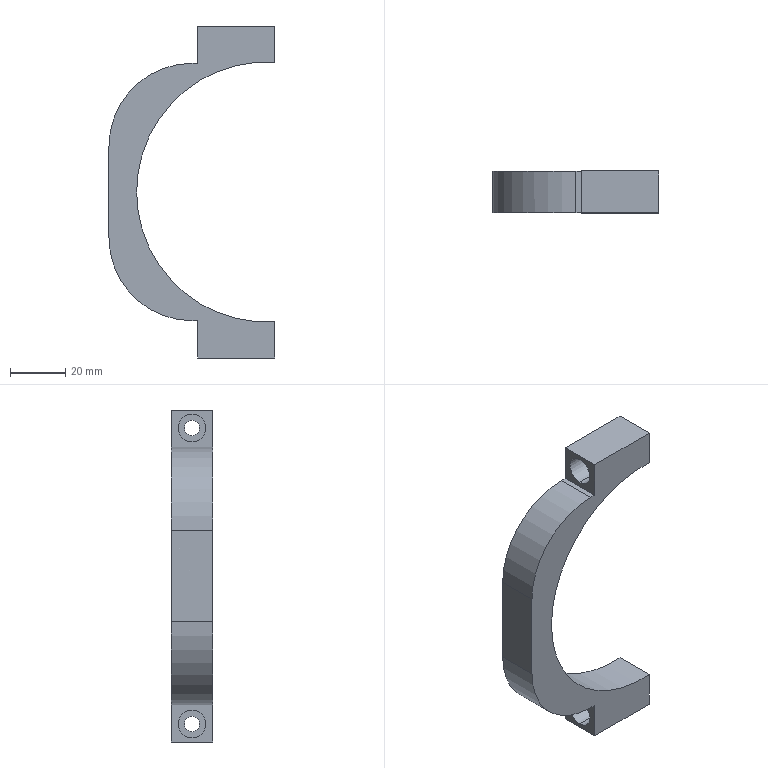Part | STEP file | 11-FG-S01311 | 1 solid | 25 faces | box 60 x 15 x 120 mm | volume 30172 mm3 | plane 13 | cylinder 12 | commonest cylinder face diameters 5.5 x4 10 x4 60 x2 94 x2
STEP:
#1=CARTESIAN_POINT('',(-14.6,7.5,1.5));
#2=VERTEX_POINT('',#1);
#3=CARTESIAN_POINT('',(-14.6,7.5,11.5));
#4=VERTEX_POINT('',#3);
#5=CARTESIAN_POINT('',(-14.6,7.5,6.5));
#6=DIRECTION('',(-1.,0.,0.));
#7=DIRECTION('',(0.,0.,1.));
#8=AXIS2_PLACEMENT_3D('',#5,#6,#7);
#9=CIRCLE('',#8,5.);
#10=EDGE_CURVE('',#2,#4,#9,.T.);
#11=ORIENTED_EDGE('',*,*,#10,.F.);
#12=CARTESIAN_POINT('',(-28.,7.5,1.5));
#13=VERTEX_POINT('',#12);
#14=CARTESIAN_POINT('',(-60.,7.5,1.5));
#15=DIRECTION('',(-1.,0.,0.));
#16=VECTOR('',#15,1000.);
#17=LINE('',#14,#16);
#18=EDGE_CURVE('',#2,#13,#17,.T.);
#19=ORIENTED_EDGE('',*,*,#18,.T.);
#20=CARTESIAN_POINT('',(-28.,7.5,11.5));
#21=VERTEX_POINT('',#20);
#22=CARTESIAN_POINT('',(-28.,7.5,6.5));
#23=DIRECTION('',(-1.,0.,0.));
#24=DIRECTION('',(0.,1.,0.));
#25=AXIS2_PLACEMENT_3D('',#22,#23,#24);
#26=CIRCLE('',#25,5.);
#27=EDGE_CURVE('',#13,#21,#26,.T.);
#28=ORIENTED_EDGE('',*,*,#27,.T.);
#29=CARTESIAN_POINT('',(-60.,7.5,11.5));
#30=DIRECTION('',(-1.,0.,0.));
#31=VECTOR('',#30,1000.);
#32=LINE('',#29,#31);
#33=EDGE_CURVE('',#4,#21,#32,.T.);
#34=ORIENTED_EDGE('',*,*,#33,.F.);
#35=EDGE_LOOP('',(#11,#19,#28,#34));
#36=FACE_OUTER_BOUND('',#35,.T.);
#37=CARTESIAN_POINT('',(-60.,7.5,6.5));
#38=DIRECTION('',(-1.,0.,0.));
#39=DIRECTION('',(0.,0.,1.));
#40=AXIS2_PLACEMENT_3D('',#37,#38,#39);
#41=CYLINDRICAL_SURFACE('',#40,5.);
#42=ADVANCED_FACE('',(#36),#41,.F.);
#43=CARTESIAN_POINT('',(0.,7.5,3.75));
#44=VERTEX_POINT('',#43);
#45=CARTESIAN_POINT('',(0.,7.5,9.25));
#46=VERTEX_POINT('',#45);
#47=CARTESIAN_POINT('',(0.,7.5,6.5));
#48=DIRECTION('',(-1.,0.,0.));
#49=DIRECTION('',(0.,0.,1.));
#50=AXIS2_PLACEMENT_3D('',#47,#48,#49);
#51=CIRCLE('',#50,2.75);
#52=EDGE_CURVE('',#44,#46,#51,.T.);
#53=ORIENTED_EDGE('',*,*,#52,.F.);
#54=CARTESIAN_POINT('',(-14.6,7.5,3.75));
#55=VERTEX_POINT('',#54);
#56=CARTESIAN_POINT('',(-60.,7.5,3.75));
#57=DIRECTION('',(-1.,0.,0.));
#58=VECTOR('',#57,1000.);
#59=LINE('',#56,#58);
#60=EDGE_CURVE('',#44,#55,#59,.T.);
#61=ORIENTED_EDGE('',*,*,#60,.T.);
#62=CARTESIAN_POINT('',(-14.6,7.5,9.25));
#63=VERTEX_POINT('',#62);
#64=CARTESIAN_POINT('',(-14.6,7.5,6.5));
#65=DIRECTION('',(-1.,0.,0.));
#66=DIRECTION('',(0.,0.,1.));
#67=AXIS2_PLACEMENT_3D('',#64,#65,#66);
#68=CIRCLE('',#67,2.75);
#69=EDGE_CURVE('',#55,#63,#68,.T.);
#70=ORIENTED_EDGE('',*,*,#69,.T.);
#71=CARTESIAN_POINT('',(-60.,7.5,9.25));
#72=DIRECTION('',(-1.,0.,0.));
#73=VECTOR('',#72,1000.);
#74=LINE('',#71,#73);
#75=EDGE_CURVE('',#46,#63,#74,.T.);
#76=ORIENTED_EDGE('',*,*,#75,.F.);
#77=EDGE_LOOP('',(#53,#61,#70,#76));
#78=FACE_OUTER_BOUND('',#77,.T.);
#79=CARTESIAN_POINT('',(-60.,7.5,6.5));
#80=DIRECTION('',(-1.,0.,0.));
#81=DIRECTION('',(0.,0.,1.));
#82=AXIS2_PLACEMENT_3D('',#79,#80,#81);
#83=CYLINDRICAL_SURFACE('',#82,2.75);
#84=ADVANCED_FACE('',(#78),#83,.F.);
#85=CARTESIAN_POINT('',(-14.6,7.5,108.5));
#86=VERTEX_POINT('',#85);
#87=CARTESIAN_POINT('',(-14.6,7.5,118.5));
#88=VERTEX_POINT('',#87);
#89=CARTESIAN_POINT('',(-14.6,7.5,113.5));
#90=DIRECTION('',(-1.,0.,0.));
#91=DIRECTION('',(0.,0.,1.));
#92=AXIS2_PLACEMENT_3D('',#89,#90,#91);
#93=CIRCLE('',#92,5.);
#94=EDGE_CURVE('',#86,#88,#93,.T.);
#95=ORIENTED_EDGE('',*,*,#94,.F.);
#96=CARTESIAN_POINT('',(-28.,7.5,108.5));
#97=VERTEX_POINT('',#96);
#98=CARTESIAN_POINT('',(-60.,7.5,108.5));
#99=DIRECTION('',(-1.,0.,0.));
#100=VECTOR('',#99,1000.);
#101=LINE('',#98,#100);
#102=EDGE_CURVE('',#86,#97,#101,.T.);
#103=ORIENTED_EDGE('',*,*,#102,.T.);
#104=CARTESIAN_POINT('',(-28.,7.5,118.5));
#105=VERTEX_POINT('',#104);
#106=CARTESIAN_POINT('',(-28.,7.5,113.5));
#107=DIRECTION('',(-1.,0.,0.));
#108=DIRECTION('',(0.,1.,0.));
#109=AXIS2_PLACEMENT_3D('',#106,#107,#108);
#110=CIRCLE('',#109,5.);
#111=EDGE_CURVE('',#97,#105,#110,.T.);
#112=ORIENTED_EDGE('',*,*,#111,.T.);
#113=CARTESIAN_POINT('',(-60.,7.5,118.5));
#114=DIRECTION('',(-1.,0.,0.));
#115=VECTOR('',#114,1000.);
#116=LINE('',#113,#115);
#117=EDGE_CURVE('',#88,#105,#116,.T.);
#118=ORIENTED_EDGE('',*,*,#117,.F.);
#119=EDGE_LOOP('',(#95,#103,#112,#118));
#120=FACE_OUTER_BOUND('',#119,.T.);
#121=CARTESIAN_POINT('',(-60.,7.5,113.5));
#122=DIRECTION('',(-1.,0.,0.));
#123=DIRECTION('',(0.,0.,1.));
#124=AXIS2_PLACEMENT_3D('',#121,#122,#123);
#125=CYLINDRICAL_SURFACE('',#124,5.);
#126=ADVANCED_FACE('',(#120),#125,.F.);
#127=CARTESIAN_POINT('',(0.,7.5,110.75));
#128=VERTEX_POINT('',#127);
#129=CARTESIAN_POINT('',(0.,7.5,116.25));
#130=VERTEX_POINT('',#129);
#131=CARTESIAN_POINT('',(0.,7.5,113.5));
#132=DIRECTION('',(-1.,0.,0.));
#133=DIRECTION('',(0.,0.,1.));
#134=AXIS2_PLACEMENT_3D('',#131,#132,#133);
#135=CIRCLE('',#134,2.75);
#136=EDGE_CURVE('',#128,#130,#135,.T.);
#137=ORIENTED_EDGE('',*,*,#136,.F.);
#138=CARTESIAN_POINT('',(-14.6,7.5,110.75));
#139=VERTEX_POINT('',#138);
#140=CARTESIAN_POINT('',(-60.,7.5,110.75));
#141=DIRECTION('',(-1.,0.,0.));
#142=VECTOR('',#141,1000.);
#143=LINE('',#140,#142);
#144=EDGE_CURVE('',#128,#139,#143,.T.);
#145=ORIENTED_EDGE('',*,*,#144,.T.);
#146=CARTESIAN_POINT('',(-14.6,7.5,116.25));
#147=VERTEX_POINT('',#146);
#148=CARTESIAN_POINT('',(-14.6,7.5,113.5));
#149=DIRECTION('',(-1.,0.,0.));
#150=DIRECTION('',(0.,0.,1.));
#151=AXIS2_PLACEMENT_3D('',#148,#149,#150);
#152=CIRCLE('',#151,2.75);
#153=EDGE_CURVE('',#139,#147,#152,.T.);
#154=ORIENTED_EDGE('',*,*,#153,.T.);
#155=CARTESIAN_POINT('',(-60.,7.5,116.25));
#156=DIRECTION('',(-1.,0.,0.));
#157=VECTOR('',#156,1000.);
#158=LINE('',#155,#157);
#159=EDGE_CURVE('',#130,#147,#158,.T.);
#160=ORIENTED_EDGE('',*,*,#159,.F.);
#161=EDGE_LOOP('',(#137,#145,#154,#160));
#162=FACE_OUTER_BOUND('',#161,.T.);
#163=CARTESIAN_POINT('',(-60.,7.5,113.5));
#164=DIRECTION('',(-1.,0.,0.));
#165=DIRECTION('',(0.,0.,1.));
#166=AXIS2_PLACEMENT_3D('',#163,#164,#165);
#167=CYLINDRICAL_SURFACE('',#166,2.75);
#168=ADVANCED_FACE('',(#162),#167,.F.);
#169=CARTESIAN_POINT('',(-50.,0.,60.));
#170=VERTEX_POINT('',#169);
#171=CARTESIAN_POINT('',(0.,0.,106.904));
#172=VERTEX_POINT('',#171);
#173=CARTESIAN_POINT('',(-3.,0.,60.));
#174=DIRECTION('',(0.,1.,0.));
#175=DIRECTION('',(-1.,0.,0.));
#176=AXIS2_PLACEMENT_3D('',#173,#174,#175);
#177=CIRCLE('',#176,47.);
#178=EDGE_CURVE('',#170,#172,#177,.T.);
#179=ORIENTED_EDGE('',*,*,#178,.F.);
#180=CARTESIAN_POINT('',(-50.,15.,60.));
#181=VERTEX_POINT('',#180);
#182=CARTESIAN_POINT('',(-50.,-65.,60.));
#183=DIRECTION('',(0.,1.,0.));
#184=VECTOR('',#183,1000.);
#185=LINE('',#182,#184);
#186=EDGE_CURVE('',#170,#181,#185,.T.);
#187=ORIENTED_EDGE('',*,*,#186,.T.);
#188=CARTESIAN_POINT('',(0.,15.,106.904));
#189=VERTEX_POINT('',#188);
#190=CARTESIAN_POINT('',(-3.,15.,60.));
#191=DIRECTION('',(0.,1.,0.));
#192=DIRECTION('',(-1.,0.,0.));
#193=AXIS2_PLACEMENT_3D('',#190,#191,#192);
#194=CIRCLE('',#193,47.);
#195=EDGE_CURVE('',#181,#189,#194,.T.);
#196=ORIENTED_EDGE('',*,*,#195,.T.);
#197=CARTESIAN_POINT('',(0.,-65.,106.904));
#198=DIRECTION('',(0.,1.,0.));
#199=VECTOR('',#198,1000.);
#200=LINE('',#197,#199);
#201=EDGE_CURVE('',#172,#189,#200,.T.);
#202=ORIENTED_EDGE('',*,*,#201,.F.);
#203=EDGE_LOOP('',(#179,#187,#196,#202));
#204=FACE_OUTER_BOUND('',#203,.T.);
#205=CARTESIAN_POINT('',(-3.,-65.,60.));
#206=DIRECTION('',(0.,1.,0.));
#207=DIRECTION('',(-1.,0.,0.));
#208=AXIS2_PLACEMENT_3D('',#205,#206,#207);
#209=CYLINDRICAL_SURFACE('',#208,47.);
#210=ADVANCED_FACE('',(#204),#209,.F.);
#211=CARTESIAN_POINT('',(0.,7.5,113.5));
#212=DIRECTION('',(-1.,0.,0.));
#213=DIRECTION('',(0.,0.,1.));
#214=AXIS2_PLACEMENT_3D('',#211,#212,#213);
#215=CIRCLE('',#214,2.75);
#216=EDGE_CURVE('',#130,#128,#215,.T.);
#217=ORIENTED_EDGE('',*,*,#216,.T.);
#218=ORIENTED_EDGE('',*,*,#136,.T.);
#219=EDGE_LOOP('',(#217,#218));
#220=FACE_BOUND('',#219,.T.);
#221=CARTESIAN_POINT('',(0.,0.,120.));
#222=VERTEX_POINT('',#221);
#223=CARTESIAN_POINT('',(0.,0.,120.));
#224=DIRECTION('',(0.,0.,-1.));
#225=VECTOR('',#224,1000.);
#226=LINE('',#223,#225);
#227=EDGE_CURVE('',#222,#172,#226,.T.);
#228=ORIENTED_EDGE('',*,*,#227,.T.);
#229=ORIENTED_EDGE('',*,*,#201,.T.);
#230=CARTESIAN_POINT('',(0.,15.,120.));
#231=VERTEX_POINT('',#230);
#232=CARTESIAN_POINT('',(0.,15.,120.));
#233=DIRECTION('',(0.,0.,-1.));
#234=VECTOR('',#233,1000.);
#235=LINE('',#232,#234);
#236=EDGE_CURVE('',#231,#189,#235,.T.);
#237=ORIENTED_EDGE('',*,*,#236,.F.);
#238=CARTESIAN_POINT('',(0.,0.,120.));
#239=DIRECTION('',(0.,1.,0.));
#240=VECTOR('',#239,1000.);
#241=LINE('',#238,#240);
#242=EDGE_CURVE('',#222,#231,#241,.T.);
#243=ORIENTED_EDGE('',*,*,#242,.F.);
#244=EDGE_LOOP('',(#228,#229,#237,#243));
#245=FACE_OUTER_BOUND('',#244,.T.);
#246=CARTESIAN_POINT('',(0.,0.,120.));
#247=DIRECTION('',(-1.,0.,0.));
#248=DIRECTION('',(0.,0.,1.));
#249=AXIS2_PLACEMENT_3D('',#246,#247,#248);
#250=PLANE('',#249);
#251=ADVANCED_FACE('',(#220,#245),#250,.F.);
#252=CARTESIAN_POINT('',(0.,7.5,6.5));
#253=DIRECTION('',(-1.,0.,0.));
#254=DIRECTION('',(0.,0.,1.));
#255=AXIS2_PLACEMENT_3D('',#252,#253,#254);
#256=CIRCLE('',#255,2.75);
#257=EDGE_CURVE('',#46,#44,#256,.T.);
#258=ORIENTED_EDGE('',*,*,#257,.T.);
#259=ORIENTED_EDGE('',*,*,#52,.T.);
#260=EDGE_LOOP('',(#258,#259));
#261=FACE_BOUND('',#260,.T.);
#262=CARTESIAN_POINT('',(0.,15.,13.096));
#263=VERTEX_POINT('',#262);
#264=CARTESIAN_POINT('',(0.,15.,0.));
#265=VERTEX_POINT('',#264);
#266=CARTESIAN_POINT('',(0.,15.,120.));
#267=DIRECTION('',(0.,0.,-1.));
#268=VECTOR('',#267,1000.);
#269=LINE('',#266,#268);
#270=EDGE_CURVE('',#263,#265,#269,.T.);
#271=ORIENTED_EDGE('',*,*,#270,.F.);
#272=CARTESIAN_POINT('',(0.,0.,13.096));
#273=VERTEX_POINT('',#272);
#274=CARTESIAN_POINT('',(0.,-65.,13.096));
#275=DIRECTION('',(0.,-1.,0.));
#276=VECTOR('',#275,1000.);
#277=LINE('',#274,#276);
#278=EDGE_CURVE('',#263,#273,#277,.T.);
#279=ORIENTED_EDGE('',*,*,#278,.T.);
#280=CARTESIAN_POINT('',(0.,0.,0.));
#281=VERTEX_POINT('',#280);
#282=CARTESIAN_POINT('',(0.,0.,120.));
#283=DIRECTION('',(0.,0.,-1.));
#284=VECTOR('',#283,1000.);
#285=LINE('',#282,#284);
#286=EDGE_CURVE('',#273,#281,#285,.T.);
#287=ORIENTED_EDGE('',*,*,#286,.T.);
#288=CARTESIAN_POINT('',(0.,0.,0.));
#289=DIRECTION('',(0.,1.,0.));
#290=VECTOR('',#289,1000.);
#291=LINE('',#288,#290);
#292=EDGE_CURVE('',#281,#265,#291,.T.);
#293=ORIENTED_EDGE('',*,*,#292,.T.);
#294=EDGE_LOOP('',(#271,#279,#287,#293));
#295=FACE_OUTER_BOUND('',#294,.T.);
#296=CARTESIAN_POINT('',(0.,0.,120.));
#297=DIRECTION('',(-1.,0.,0.));
#298=DIRECTION('',(0.,0.,1.));
#299=AXIS2_PLACEMENT_3D('',#296,#297,#298);
#300=PLANE('',#299);
#301=ADVANCED_FACE('',(#261,#295),#300,.F.);
#302=CARTESIAN_POINT('',(-60.,15.,76.5));
#303=VERTEX_POINT('',#302);
#304=CARTESIAN_POINT('',(-60.,15.,43.5));
#305=VERTEX_POINT('',#304);
#306=CARTESIAN_POINT('',(-60.,15.,120.));
#307=DIRECTION('',(0.,0.,-1.));
#308=VECTOR('',#307,1000.);
#309=LINE('',#306,#308);
#310=EDGE_CURVE('',#303,#305,#309,.T.);
#311=ORIENTED_EDGE('',*,*,#310,.F.);
#312=CARTESIAN_POINT('',(-30.,15.,106.5));
#313=VERTEX_POINT('',#312);
#314=CARTESIAN_POINT('',(-30.,15.,76.5));
#315=DIRECTION('',(0.,1.,0.));
#316=DIRECTION('',(1.,0.,0.));
#317=AXIS2_PLACEMENT_3D('',#314,#315,#316);
#318=CIRCLE('',#317,30.);
#319=EDGE_CURVE('',#303,#313,#318,.T.);
#320=ORIENTED_EDGE('',*,*,#319,.T.);
#321=CARTESIAN_POINT('',(-28.,15.,106.5));
#322=VERTEX_POINT('',#321);
#323=CARTESIAN_POINT('',(0.,15.,106.5));
#324=DIRECTION('',(1.,0.,0.));
#325=VECTOR('',#324,1000.);
#326=LINE('',#323,#325);
#327=EDGE_CURVE('',#313,#322,#326,.T.);
#328=ORIENTED_EDGE('',*,*,#327,.T.);
#329=CARTESIAN_POINT('',(-28.,15.,120.));
#330=VERTEX_POINT('',#329);
#331=CARTESIAN_POINT('',(-28.,15.,120.));
#332=DIRECTION('',(0.,0.,1.));
#333=VECTOR('',#332,1000.);
#334=LINE('',#331,#333);
#335=EDGE_CURVE('',#322,#330,#334,.T.);
#336=ORIENTED_EDGE('',*,*,#335,.T.);
#337=CARTESIAN_POINT('',(0.,15.,120.));
#338=DIRECTION('',(-1.,0.,0.));
#339=VECTOR('',#338,1000.);
#340=LINE('',#337,#339);
#341=EDGE_CURVE('',#231,#330,#340,.T.);
#342=ORIENTED_EDGE('',*,*,#341,.F.);
#343=ORIENTED_EDGE('',*,*,#236,.T.);
#344=ORIENTED_EDGE('',*,*,#195,.F.);
#345=CARTESIAN_POINT('',(-3.,15.,60.));
#346=DIRECTION('',(0.,1.,0.));
#347=DIRECTION('',(-1.,0.,0.));
#348=AXIS2_PLACEMENT_3D('',#345,#346,#347);
#349=CIRCLE('',#348,47.);
#350=EDGE_CURVE('',#263,#181,#349,.T.);
#351=ORIENTED_EDGE('',*,*,#350,.F.);
#352=ORIENTED_EDGE('',*,*,#270,.T.);
#353=CARTESIAN_POINT('',(-28.,15.,0.));
#354=VERTEX_POINT('',#353);
#355=CARTESIAN_POINT('',(0.,15.,0.));
#356=DIRECTION('',(-1.,0.,0.));
#357=VECTOR('',#356,1000.);
#358=LINE('',#355,#357);
#359=EDGE_CURVE('',#265,#354,#358,.T.);
#360=ORIENTED_EDGE('',*,*,#359,.T.);
#361=CARTESIAN_POINT('',(-28.,15.,13.5));
#362=VERTEX_POINT('',#361);
#363=CARTESIAN_POINT('',(-28.,15.,120.));
#364=DIRECTION('',(0.,0.,1.));
#365=VECTOR('',#364,1000.);
#366=LINE('',#363,#365);
#367=EDGE_CURVE('',#354,#362,#366,.T.);
#368=ORIENTED_EDGE('',*,*,#367,.T.);
#369=CARTESIAN_POINT('',(-30.,15.,13.5));
#370=VERTEX_POINT('',#369);
#371=CARTESIAN_POINT('',(0.,15.,13.5));
#372=DIRECTION('',(-1.,0.,0.));
#373=VECTOR('',#372,1000.);
#374=LINE('',#371,#373);
#375=EDGE_CURVE('',#362,#370,#374,.T.);
#376=ORIENTED_EDGE('',*,*,#375,.T.);
#377=CARTESIAN_POINT('',(-30.,15.,43.5));
#378=DIRECTION('',(0.,1.,0.));
#379=DIRECTION('',(1.,0.,0.));
#380=AXIS2_PLACEMENT_3D('',#377,#378,#379);
#381=CIRCLE('',#380,30.);
#382=EDGE_CURVE('',#370,#305,#381,.T.);
#383=ORIENTED_EDGE('',*,*,#382,.T.);
#384=EDGE_LOOP('',(#311,#320,#328,#336,#342,#343,#344,#351,#352,#360,#368,#376,#383));
#385=FACE_OUTER_BOUND('',#384,.T.);
#386=CARTESIAN_POINT('',(0.,15.,120.));
#387=DIRECTION('',(0.,-1.,0.));
#388=DIRECTION('',(1.,0.,0.));
#389=AXIS2_PLACEMENT_3D('',#386,#387,#388);
#390=PLANE('',#389);
#391=ADVANCED_FACE('',(#385),#390,.F.);
#392=CARTESIAN_POINT('',(-60.,0.,76.5));
#393=VERTEX_POINT('',#392);
#394=CARTESIAN_POINT('',(-60.,0.,43.5));
#395=VERTEX_POINT('',#394);
#396=CARTESIAN_POINT('',(-60.,0.,120.));
#397=DIRECTION('',(0.,0.,-1.));
#398=VECTOR('',#397,1000.);
#399=LINE('',#396,#398);
#400=EDGE_CURVE('',#393,#395,#399,.T.);
#401=ORIENTED_EDGE('',*,*,#400,.F.);
#402=CARTESIAN_POINT('',(-60.,0.,76.5));
#403=DIRECTION('',(0.,1.,0.));
#404=VECTOR('',#403,1000.);
#405=LINE('',#402,#404);
#406=EDGE_CURVE('',#393,#303,#405,.T.);
#407=ORIENTED_EDGE('',*,*,#406,.T.);
#408=ORIENTED_EDGE('',*,*,#310,.T.);
#409=CARTESIAN_POINT('',(-60.,0.,43.5));
#410=DIRECTION('',(0.,-1.,0.));
#411=VECTOR('',#410,1000.);
#412=LINE('',#409,#411);
#413=EDGE_CURVE('',#305,#395,#412,.T.);
#414=ORIENTED_EDGE('',*,*,#413,.T.);
#415=EDGE_LOOP('',(#401,#407,#408,#414));
#416=FACE_OUTER_BOUND('',#415,.T.);
#417=CARTESIAN_POINT('',(-60.,0.,120.));
#418=DIRECTION('',(1.,0.,0.));
#419=DIRECTION('',(0.,0.,-1.));
#420=AXIS2_PLACEMENT_3D('',#417,#418,#419);
#421=PLANE('',#420);
#422=ADVANCED_FACE('',(#416),#421,.F.);
#423=CARTESIAN_POINT('',(-30.,0.,106.5));
#424=VERTEX_POINT('',#423);
#425=CARTESIAN_POINT('',(-28.,0.,106.5));
#426=VERTEX_POINT('',#425);
#427=CARTESIAN_POINT('',(-60.,0.,106.5));
#428=DIRECTION('',(1.,0.,0.));
#429=VECTOR('',#428,1000.);
#430=LINE('',#427,#429);
#431=EDGE_CURVE('',#424,#426,#430,.T.);
#432=ORIENTED_EDGE('',*,*,#431,.F.);
#433=CARTESIAN_POINT('',(-30.,0.,76.5));
#434=DIRECTION('',(0.,-1.,0.));
#435=DIRECTION('',(-1.,0.,0.));
#436=AXIS2_PLACEMENT_3D('',#433,#434,#435);
#437=CIRCLE('',#436,30.);
#438=EDGE_CURVE('',#424,#393,#437,.T.);
#439=ORIENTED_EDGE('',*,*,#438,.T.);
#440=ORIENTED_EDGE('',*,*,#400,.T.);
#441=CARTESIAN_POINT('',(-30.,0.,13.5));
#442=VERTEX_POINT('',#441);
#443=CARTESIAN_POINT('',(-30.,0.,43.5));
#444=DIRECTION('',(0.,-1.,0.));
#445=DIRECTION('',(-1.,0.,0.));
#446=AXIS2_PLACEMENT_3D('',#443,#444,#445);
#447=CIRCLE('',#446,30.);
#448=EDGE_CURVE('',#395,#442,#447,.T.);
#449=ORIENTED_EDGE('',*,*,#448,.T.);
#450=CARTESIAN_POINT('',(-28.,0.,13.5));
#451=VERTEX_POINT('',#450);
#452=CARTESIAN_POINT('',(-60.,0.,13.5));
#453=DIRECTION('',(-1.,0.,0.));
#454=VECTOR('',#453,1000.);
#455=LINE('',#452,#454);
#456=EDGE_CURVE('',#451,#442,#455,.T.);
#457=ORIENTED_EDGE('',*,*,#456,.F.);
#458=CARTESIAN_POINT('',(-28.,0.,0.));
#459=VERTEX_POINT('',#458);
#460=CARTESIAN_POINT('',(-28.,0.,0.));
#461=DIRECTION('',(0.,0.,1.));
#462=VECTOR('',#461,1000.);
#463=LINE('',#460,#462);
#464=EDGE_CURVE('',#459,#451,#463,.T.);
#465=ORIENTED_EDGE('',*,*,#464,.F.);
#466=CARTESIAN_POINT('',(0.,0.,0.));
#467=DIRECTION('',(1.,0.,0.));
#468=VECTOR('',#467,1000.);
#469=LINE('',#466,#468);
#470=EDGE_CURVE('',#459,#281,#469,.T.);
#471=ORIENTED_EDGE('',*,*,#470,.T.);
#472=ORIENTED_EDGE('',*,*,#286,.F.);
#473=CARTESIAN_POINT('',(-3.,0.,60.));
#474=DIRECTION('',(0.,1.,0.));
#475=DIRECTION('',(-1.,0.,0.));
#476=AXIS2_PLACEMENT_3D('',#473,#474,#475);
#477=CIRCLE('',#476,47.);
#478=EDGE_CURVE('',#273,#170,#477,.T.);
#479=ORIENTED_EDGE('',*,*,#478,.T.);
#480=ORIENTED_EDGE('',*,*,#178,.T.);
#481=ORIENTED_EDGE('',*,*,#227,.F.);
#482=CARTESIAN_POINT('',(-28.,0.,120.));
#483=VERTEX_POINT('',#482);
#484=CARTESIAN_POINT('',(0.,0.,120.));
#485=DIRECTION('',(1.,0.,0.));
#486=VECTOR('',#485,1000.);
#487=LINE('',#484,#486);
#488=EDGE_CURVE('',#483,#222,#487,.T.);
#489=ORIENTED_EDGE('',*,*,#488,.F.);
#490=CARTESIAN_POINT('',(-28.,0.,120.));
#491=DIRECTION('',(0.,0.,1.));
#492=VECTOR('',#491,1000.);
#493=LINE('',#490,#492);
#494=EDGE_CURVE('',#426,#483,#493,.T.);
#495=ORIENTED_EDGE('',*,*,#494,.F.);
#496=EDGE_LOOP('',(#432,#439,#440,#449,#457,#465,#471,#472,#479,#480,#481,#489,#495));
#497=FACE_OUTER_BOUND('',#496,.T.);
#498=CARTESIAN_POINT('',(0.,0.,120.));
#499=DIRECTION('',(0.,1.,0.));
#500=DIRECTION('',(-1.,0.,0.));
#501=AXIS2_PLACEMENT_3D('',#498,#499,#500);
#502=PLANE('',#501);
#503=ADVANCED_FACE('',(#497),#502,.F.);
#504=CARTESIAN_POINT('',(-28.,42.,120.));
#505=DIRECTION('',(0.,-1.,0.));
#506=VECTOR('',#505,1000.);
#507=LINE('',#504,#506);
#508=EDGE_CURVE('',#330,#483,#507,.T.);
#509=ORIENTED_EDGE('',*,*,#508,.T.);
#510=ORIENTED_EDGE('',*,*,#488,.T.);
#511=ORIENTED_EDGE('',*,*,#242,.T.);
#512=ORIENTED_EDGE('',*,*,#341,.T.);
#513=EDGE_LOOP('',(#509,#510,#511,#512));
#514=FACE_OUTER_BOUND('',#513,.T.);
#515=CARTESIAN_POINT('',(0.,15.,120.));
#516=DIRECTION('',(0.,0.,1.));
#517=DIRECTION('',(1.,0.,0.));
#518=AXIS2_PLACEMENT_3D('',#515,#516,#517);
#519=PLANE('',#518);
#520=ADVANCED_FACE('',(#514),#519,.T.);
#521=ORIENTED_EDGE('',*,*,#470,.F.);
#522=CARTESIAN_POINT('',(-28.,42.,0.));
#523=DIRECTION('',(0.,-1.,0.));
#524=VECTOR('',#523,1000.);
#525=LINE('',#522,#524);
#526=EDGE_CURVE('',#354,#459,#525,.T.);
#527=ORIENTED_EDGE('',*,*,#526,.F.);
#528=ORIENTED_EDGE('',*,*,#359,.F.);
#529=ORIENTED_EDGE('',*,*,#292,.F.);
#530=EDGE_LOOP('',(#521,#527,#528,#529));
#531=FACE_OUTER_BOUND('',#530,.T.);
#532=CARTESIAN_POINT('',(0.,15.,0.));
#533=DIRECTION('',(0.,0.,1.));
#534=DIRECTION('',(1.,0.,0.));
#535=AXIS2_PLACEMENT_3D('',#532,#533,#534);
#536=PLANE('',#535);
#537=ADVANCED_FACE('',(#531),#536,.F.);
#538=ORIENTED_EDGE('',*,*,#186,.F.);
#539=ORIENTED_EDGE('',*,*,#478,.F.);
#540=ORIENTED_EDGE('',*,*,#278,.F.);
#541=ORIENTED_EDGE('',*,*,#350,.T.);
#542=EDGE_LOOP('',(#538,#539,#540,#541));
#543=FACE_OUTER_BOUND('',#542,.T.);
#544=CARTESIAN_POINT('',(-3.,-65.,60.));
#545=DIRECTION('',(0.,1.,0.));
#546=DIRECTION('',(-1.,0.,0.));
#547=AXIS2_PLACEMENT_3D('',#544,#545,#546);
#548=CYLINDRICAL_SURFACE('',#547,47.);
#549=ADVANCED_FACE('',(#543),#548,.F.);
#550=ORIENTED_EDGE('',*,*,#144,.F.);
#551=ORIENTED_EDGE('',*,*,#216,.F.);
#552=ORIENTED_EDGE('',*,*,#159,.T.);
#553=CARTESIAN_POINT('',(-14.6,7.5,113.5));
#554=DIRECTION('',(-1.,0.,0.));
#555=DIRECTION('',(0.,0.,1.));
#556=AXIS2_PLACEMENT_3D('',#553,#554,#555);
#557=CIRCLE('',#556,2.75);
#558=EDGE_CURVE('',#147,#139,#557,.T.);
#559=ORIENTED_EDGE('',*,*,#558,.T.);
#560=EDGE_LOOP('',(#550,#551,#552,#559));
#561=FACE_OUTER_BOUND('',#560,.T.);
#562=CARTESIAN_POINT('',(-60.,7.5,113.5));
#563=DIRECTION('',(-1.,0.,0.));
#564=DIRECTION('',(0.,0.,1.));
#565=AXIS2_PLACEMENT_3D('',#562,#563,#564);
#566=CYLINDRICAL_SURFACE('',#565,2.75);
#567=ADVANCED_FACE('',(#561),#566,.F.);
#568=ORIENTED_EDGE('',*,*,#558,.F.);
#569=ORIENTED_EDGE('',*,*,#153,.F.);
#570=EDGE_LOOP('',(#568,#569));
#571=FACE_BOUND('',#570,.T.);
#572=CARTESIAN_POINT('',(-14.6,7.5,113.5));
#573=DIRECTION('',(-1.,0.,0.));
#574=DIRECTION('',(0.,0.,1.));
#575=AXIS2_PLACEMENT_3D('',#572,#573,#574);
#576=CIRCLE('',#575,5.);
#577=EDGE_CURVE('',#88,#86,#576,.T.);
#578=ORIENTED_EDGE('',*,*,#577,.T.);
#579=ORIENTED_EDGE('',*,*,#94,.T.);
#580=EDGE_LOOP('',(#578,#579));
#581=FACE_OUTER_BOUND('',#580,.T.);
#582=CARTESIAN_POINT('',(-14.6,10.25,113.5));
#583=DIRECTION('',(1.,0.,0.));
#584=DIRECTION('',(0.,0.,-1.));
#585=AXIS2_PLACEMENT_3D('',#582,#583,#584);
#586=PLANE('',#585);
#587=ADVANCED_FACE('',(#571,#581),#586,.F.);
#588=ORIENTED_EDGE('',*,*,#102,.F.);
#589=ORIENTED_EDGE('',*,*,#577,.F.);
#590=ORIENTED_EDGE('',*,*,#117,.T.);
#591=CARTESIAN_POINT('',(-28.,7.5,113.5));
#592=DIRECTION('',(-1.,0.,0.));
#593=DIRECTION('',(0.,1.,0.));
#594=AXIS2_PLACEMENT_3D('',#591,#592,#593);
#595=CIRCLE('',#594,5.);
#596=EDGE_CURVE('',#105,#97,#595,.T.);
#597=ORIENTED_EDGE('',*,*,#596,.T.);
#598=EDGE_LOOP('',(#588,#589,#590,#597));
#599=FACE_OUTER_BOUND('',#598,.T.);
#600=CARTESIAN_POINT('',(-60.,7.5,113.5));
#601=DIRECTION('',(-1.,0.,0.));
#602=DIRECTION('',(0.,0.,1.));
#603=AXIS2_PLACEMENT_3D('',#600,#601,#602);
#604=CYLINDRICAL_SURFACE('',#603,5.);
#605=ADVANCED_FACE('',(#599),#604,.F.);
#606=ORIENTED_EDGE('',*,*,#60,.F.);
#607=ORIENTED_EDGE('',*,*,#257,.F.);
#608=ORIENTED_EDGE('',*,*,#75,.T.);
#609=CARTESIAN_POINT('',(-14.6,7.5,6.5));
#610=DIRECTION('',(-1.,0.,0.));
#611=DIRECTION('',(0.,0.,1.));
#612=AXIS2_PLACEMENT_3D('',#609,#610,#611);
#613=CIRCLE('',#612,2.75);
#614=EDGE_CURVE('',#63,#55,#613,.T.);
#615=ORIENTED_EDGE('',*,*,#614,.T.);
#616=EDGE_LOOP('',(#606,#607,#608,#615));
#617=FACE_OUTER_BOUND('',#616,.T.);
#618=CARTESIAN_POINT('',(-60.,7.5,6.5));
#619=DIRECTION('',(-1.,0.,0.));
#620=DIRECTION('',(0.,0.,1.));
#621=AXIS2_PLACEMENT_3D('',#618,#619,#620);
#622=CYLINDRICAL_SURFACE('',#621,2.75);
#623=ADVANCED_FACE('',(#617),#622,.F.);
#624=ORIENTED_EDGE('',*,*,#614,.F.);
#625=ORIENTED_EDGE('',*,*,#69,.F.);
#626=EDGE_LOOP('',(#624,#625));
#627=FACE_BOUND('',#626,.T.);
#628=CARTESIAN_POINT('',(-14.6,7.5,6.5));
#629=DIRECTION('',(-1.,0.,0.));
#630=DIRECTION('',(0.,0.,1.));
#631=AXIS2_PLACEMENT_3D('',#628,#629,#630);
#632=CIRCLE('',#631,5.);
#633=EDGE_CURVE('',#4,#2,#632,.T.);
#634=ORIENTED_EDGE('',*,*,#633,.T.);
#635=ORIENTED_EDGE('',*,*,#10,.T.);
#636=EDGE_LOOP('',(#634,#635));
#637=FACE_OUTER_BOUND('',#636,.T.);
#638=CARTESIAN_POINT('',(-14.6,10.25,6.5));
#639=DIRECTION('',(1.,0.,0.));
#640=DIRECTION('',(0.,0.,-1.));
#641=AXIS2_PLACEMENT_3D('',#638,#639,#640);
#642=PLANE('',#641);
#643=ADVANCED_FACE('',(#627,#637),#642,.F.);
#644=ORIENTED_EDGE('',*,*,#18,.F.);
#645=ORIENTED_EDGE('',*,*,#633,.F.);
#646=ORIENTED_EDGE('',*,*,#33,.T.);
#647=CARTESIAN_POINT('',(-28.,7.5,6.5));
#648=DIRECTION('',(-1.,0.,0.));
#649=DIRECTION('',(0.,1.,0.));
#650=AXIS2_PLACEMENT_3D('',#647,#648,#649);
#651=CIRCLE('',#650,5.);
#652=EDGE_CURVE('',#21,#13,#651,.T.);
#653=ORIENTED_EDGE('',*,*,#652,.T.);
#654=EDGE_LOOP('',(#644,#645,#646,#653));
#655=FACE_OUTER_BOUND('',#654,.T.);
#656=CARTESIAN_POINT('',(-60.,7.5,6.5));
#657=DIRECTION('',(-1.,0.,0.));
#658=DIRECTION('',(0.,0.,1.));
#659=AXIS2_PLACEMENT_3D('',#656,#657,#658);
#660=CYLINDRICAL_SURFACE('',#659,5.);
#661=ADVANCED_FACE('',(#655),#660,.F.);
#662=ORIENTED_EDGE('',*,*,#456,.T.);
#663=CARTESIAN_POINT('',(-30.,42.,13.5));
#664=DIRECTION('',(0.,1.,0.));
#665=VECTOR('',#664,1000.);
#666=LINE('',#663,#665);
#667=EDGE_CURVE('',#442,#370,#666,.T.);
#668=ORIENTED_EDGE('',*,*,#667,.T.);
#669=ORIENTED_EDGE('',*,*,#375,.F.);
#670=CARTESIAN_POINT('',(-28.,42.,13.5));
#671=DIRECTION('',(0.,-1.,0.));
#672=VECTOR('',#671,1000.);
#673=LINE('',#670,#672);
#674=EDGE_CURVE('',#362,#451,#673,.T.);
#675=ORIENTED_EDGE('',*,*,#674,.T.);
#676=EDGE_LOOP('',(#662,#668,#669,#675));
#677=FACE_OUTER_BOUND('',#676,.T.);
#678=CARTESIAN_POINT('',(-60.,42.,13.5));
#679=DIRECTION('',(0.,0.,1.));
#680=DIRECTION('',(1.,0.,0.));
#681=AXIS2_PLACEMENT_3D('',#678,#679,#680);
#682=PLANE('',#681);
#683=ADVANCED_FACE('',(#677),#682,.F.);
#684=ORIENTED_EDGE('',*,*,#652,.F.);
#685=ORIENTED_EDGE('',*,*,#27,.F.);
#686=EDGE_LOOP('',(#684,#685));
#687=FACE_BOUND('',#686,.T.);
#688=ORIENTED_EDGE('',*,*,#526,.T.);
#689=ORIENTED_EDGE('',*,*,#464,.T.);
#690=ORIENTED_EDGE('',*,*,#674,.F.);
#691=ORIENTED_EDGE('',*,*,#367,.F.);
#692=EDGE_LOOP('',(#688,#689,#690,#691));
#693=FACE_OUTER_BOUND('',#692,.T.);
#694=CARTESIAN_POINT('',(-28.,42.,0.));
#695=DIRECTION('',(1.,0.,0.));
#696=DIRECTION('',(0.,1.,0.));
#697=AXIS2_PLACEMENT_3D('',#694,#695,#696);
#698=PLANE('',#697);
#699=ADVANCED_FACE('',(#687,#693),#698,.F.);
#700=ORIENTED_EDGE('',*,*,#327,.F.);
#701=CARTESIAN_POINT('',(-30.,42.,106.5));
#702=DIRECTION('',(0.,-1.,0.));
#703=VECTOR('',#702,1000.);
#704=LINE('',#701,#703);
#705=EDGE_CURVE('',#313,#424,#704,.T.);
#706=ORIENTED_EDGE('',*,*,#705,.T.);
#707=ORIENTED_EDGE('',*,*,#431,.T.);
#708=CARTESIAN_POINT('',(-28.,42.,106.5));
#709=DIRECTION('',(0.,-1.,0.));
#710=VECTOR('',#709,1000.);
#711=LINE('',#708,#710);
#712=EDGE_CURVE('',#322,#426,#711,.T.);
#713=ORIENTED_EDGE('',*,*,#712,.F.);
#714=EDGE_LOOP('',(#700,#706,#707,#713));
#715=FACE_OUTER_BOUND('',#714,.T.);
#716=CARTESIAN_POINT('',(-60.,42.,106.5));
#717=DIRECTION('',(0.,0.,-1.));
#718=DIRECTION('',(-1.,0.,0.));
#719=AXIS2_PLACEMENT_3D('',#716,#717,#718);
#720=PLANE('',#719);
#721=ADVANCED_FACE('',(#715),#720,.F.);
#722=ORIENTED_EDGE('',*,*,#596,.F.);
#723=ORIENTED_EDGE('',*,*,#111,.F.);
#724=EDGE_LOOP('',(#722,#723));
#725=FACE_BOUND('',#724,.T.);
#726=ORIENTED_EDGE('',*,*,#712,.T.);
#727=ORIENTED_EDGE('',*,*,#494,.T.);
#728=ORIENTED_EDGE('',*,*,#508,.F.);
#729=ORIENTED_EDGE('',*,*,#335,.F.);
#730=EDGE_LOOP('',(#726,#727,#728,#729));
#731=FACE_OUTER_BOUND('',#730,.T.);
#732=CARTESIAN_POINT('',(-28.,42.,120.));
#733=DIRECTION('',(1.,0.,0.));
#734=DIRECTION('',(0.,1.,0.));
#735=AXIS2_PLACEMENT_3D('',#732,#733,#734);
#736=PLANE('',#735);
#737=ADVANCED_FACE('',(#725,#731),#736,.F.);
#738=ORIENTED_EDGE('',*,*,#319,.F.);
#739=ORIENTED_EDGE('',*,*,#406,.F.);
#740=ORIENTED_EDGE('',*,*,#438,.F.);
#741=ORIENTED_EDGE('',*,*,#705,.F.);
#742=EDGE_LOOP('',(#738,#739,#740,#741));
#743=FACE_OUTER_BOUND('',#742,.T.);
#744=CARTESIAN_POINT('',(-30.,42.,76.5));
#745=DIRECTION('',(0.,-1.,0.));
#746=DIRECTION('',(0.,0.,-1.));
#747=AXIS2_PLACEMENT_3D('',#744,#745,#746);
#748=CYLINDRICAL_SURFACE('',#747,30.);
#749=ADVANCED_FACE('',(#743),#748,.T.);
#750=ORIENTED_EDGE('',*,*,#382,.F.);
#751=ORIENTED_EDGE('',*,*,#667,.F.);
#752=ORIENTED_EDGE('',*,*,#448,.F.);
#753=ORIENTED_EDGE('',*,*,#413,.F.);
#754=EDGE_LOOP('',(#750,#751,#752,#753));
#755=FACE_OUTER_BOUND('',#754,.T.);
#756=CARTESIAN_POINT('',(-30.,0.,43.5));
#757=DIRECTION('',(0.,-1.,0.));
#758=DIRECTION('',(0.,0.,-1.));
#759=AXIS2_PLACEMENT_3D('',#756,#757,#758);
#760=CYLINDRICAL_SURFACE('',#759,30.);
#761=ADVANCED_FACE('',(#755),#760,.T.);
#762=CLOSED_SHELL('',(#42,#84,#126,#168,#210,#251,#301,#391,#422,#503,#520,#537,#549,#567,#587,#605,#623,#643,#661,#683,#699,#721,#737,#749,#761));
#763=MANIFOLD_SOLID_BREP('',#762);
#764=CARTESIAN_POINT('',(0.,0.,0.));
#765=DIRECTION('',(0.,0.,1.));
#766=DIRECTION('',(1.,0.,0.));
#767=AXIS2_PLACEMENT_3D('',#764,#765,#766);
#768=(LENGTH_UNIT()NAMED_UNIT(*)SI_UNIT(.MILLI.,.METRE.));
#769=UNCERTAINTY_MEASURE_WITH_UNIT(LENGTH_MEASURE(0.00001),#768,'','');
#770=(NAMED_UNIT(*)PLANE_ANGLE_UNIT()SI_UNIT($,.RADIAN.));
#771=(NAMED_UNIT(*)SI_UNIT($,.STERADIAN.)SOLID_ANGLE_UNIT());
#772=(GEOMETRIC_REPRESENTATION_CONTEXT(3)GLOBAL_UNCERTAINTY_ASSIGNED_CONTEXT((#769))GLOBAL_UNIT_ASSIGNED_CONTEXT((#768,#770,#771))REPRESENTATION_CONTEXT('',''));
#773=ADVANCED_BREP_SHAPE_REPRESENTATION('',(#763,#767),#772);